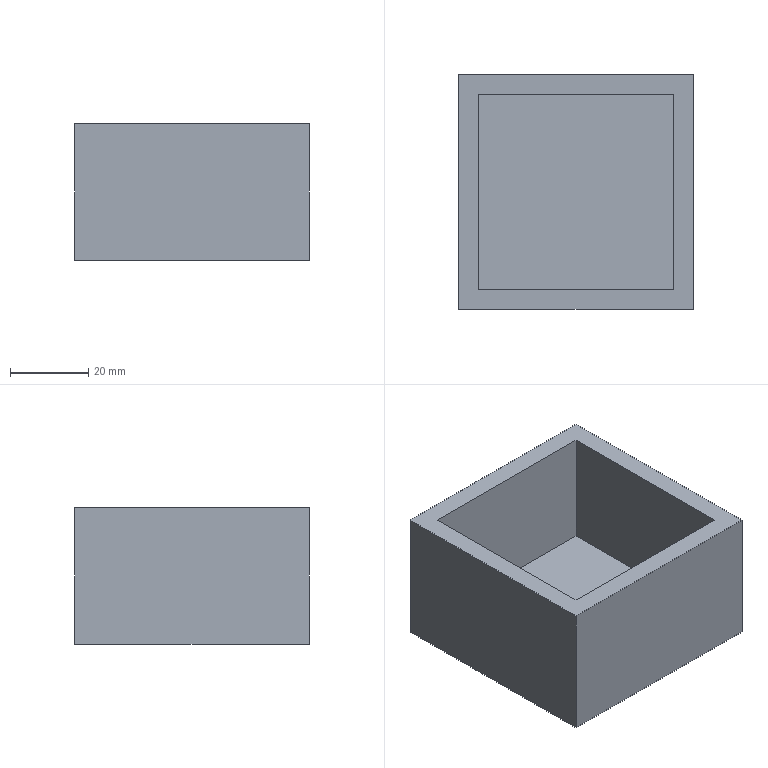Part | SolidWorks | features Extrusion 1, Shell 1 | 1 solid | 11 faces | box 60 x 60 x 35 mm | volume 51000 mm3 | plane 11
STEP:
#1=CARTESIAN_POINT('',(-58.,-30.,0.));
#2=VERTEX_POINT('',#1);
#3=CARTESIAN_POINT('',(-58.,30.,0.));
#4=VERTEX_POINT('',#3);
#5=CARTESIAN_POINT('',(-58.,30.,0.));
#6=DIRECTION('',(0.,1.,0.));
#7=VECTOR('',#6,1000.);
#8=LINE('',#5,#7);
#9=EDGE_CURVE('',#2,#4,#8,.T.);
#10=ORIENTED_EDGE('',*,*,#9,.T.);
#11=CARTESIAN_POINT('',(-58.,30.,35.));
#12=VERTEX_POINT('',#11);
#13=CARTESIAN_POINT('',(-58.,30.,35.));
#14=DIRECTION('',(0.,0.,-1.));
#15=VECTOR('',#14,1000.);
#16=LINE('',#13,#15);
#17=EDGE_CURVE('',#12,#4,#16,.T.);
#18=ORIENTED_EDGE('',*,*,#17,.F.);
#19=CARTESIAN_POINT('',(-58.,-30.,35.));
#20=VERTEX_POINT('',#19);
#21=CARTESIAN_POINT('',(-58.,30.,35.));
#22=DIRECTION('',(0.,1.,0.));
#23=VECTOR('',#22,1000.);
#24=LINE('',#21,#23);
#25=EDGE_CURVE('',#20,#12,#24,.T.);
#26=ORIENTED_EDGE('',*,*,#25,.F.);
#27=CARTESIAN_POINT('',(-58.,-30.,35.));
#28=DIRECTION('',(0.,0.,-1.));
#29=VECTOR('',#28,1000.);
#30=LINE('',#27,#29);
#31=EDGE_CURVE('',#20,#2,#30,.T.);
#32=ORIENTED_EDGE('',*,*,#31,.T.);
#33=EDGE_LOOP('',(#10,#18,#26,#32));
#34=FACE_OUTER_BOUND('',#33,.T.);
#35=CARTESIAN_POINT('',(-58.,30.,35.));
#36=DIRECTION('',(-1.,0.,0.));
#37=DIRECTION('',(0.,-1.,0.));
#38=AXIS2_PLACEMENT_3D('',#35,#36,#37);
#39=PLANE('',#38);
#40=ADVANCED_FACE('',(#34),#39,.F.);
#41=CARTESIAN_POINT('',(-118.,30.,0.));
#42=VERTEX_POINT('',#41);
#43=CARTESIAN_POINT('',(-118.,30.,0.));
#44=DIRECTION('',(-1.,0.,0.));
#45=VECTOR('',#44,1000.);
#46=LINE('',#43,#45);
#47=EDGE_CURVE('',#4,#42,#46,.T.);
#48=ORIENTED_EDGE('',*,*,#47,.T.);
#49=CARTESIAN_POINT('',(-118.,30.,35.));
#50=VERTEX_POINT('',#49);
#51=CARTESIAN_POINT('',(-118.,30.,35.));
#52=DIRECTION('',(0.,0.,-1.));
#53=VECTOR('',#52,1000.);
#54=LINE('',#51,#53);
#55=EDGE_CURVE('',#50,#42,#54,.T.);
#56=ORIENTED_EDGE('',*,*,#55,.F.);
#57=CARTESIAN_POINT('',(-118.,30.,35.));
#58=DIRECTION('',(-1.,0.,0.));
#59=VECTOR('',#58,1000.);
#60=LINE('',#57,#59);
#61=EDGE_CURVE('',#12,#50,#60,.T.);
#62=ORIENTED_EDGE('',*,*,#61,.F.);
#63=ORIENTED_EDGE('',*,*,#17,.T.);
#64=EDGE_LOOP('',(#48,#56,#62,#63));
#65=FACE_OUTER_BOUND('',#64,.T.);
#66=CARTESIAN_POINT('',(-118.,30.,35.));
#67=DIRECTION('',(0.,-1.,0.));
#68=DIRECTION('',(0.,0.,-1.));
#69=AXIS2_PLACEMENT_3D('',#66,#67,#68);
#70=PLANE('',#69);
#71=ADVANCED_FACE('',(#65),#70,.F.);
#72=CARTESIAN_POINT('',(-118.,-30.,0.));
#73=VERTEX_POINT('',#72);
#74=CARTESIAN_POINT('',(-118.,30.,0.));
#75=DIRECTION('',(0.,-1.,0.));
#76=VECTOR('',#75,1000.);
#77=LINE('',#74,#76);
#78=EDGE_CURVE('',#42,#73,#77,.T.);
#79=ORIENTED_EDGE('',*,*,#78,.T.);
#80=CARTESIAN_POINT('',(-118.,-30.,35.));
#81=VERTEX_POINT('',#80);
#82=CARTESIAN_POINT('',(-118.,-30.,35.));
#83=DIRECTION('',(0.,0.,-1.));
#84=VECTOR('',#83,1000.);
#85=LINE('',#82,#84);
#86=EDGE_CURVE('',#81,#73,#85,.T.);
#87=ORIENTED_EDGE('',*,*,#86,.F.);
#88=CARTESIAN_POINT('',(-118.,30.,35.));
#89=DIRECTION('',(0.,-1.,0.));
#90=VECTOR('',#89,1000.);
#91=LINE('',#88,#90);
#92=EDGE_CURVE('',#50,#81,#91,.T.);
#93=ORIENTED_EDGE('',*,*,#92,.F.);
#94=ORIENTED_EDGE('',*,*,#55,.T.);
#95=EDGE_LOOP('',(#79,#87,#93,#94));
#96=FACE_OUTER_BOUND('',#95,.T.);
#97=CARTESIAN_POINT('',(-118.,30.,35.));
#98=DIRECTION('',(1.,0.,0.));
#99=DIRECTION('',(0.,1.,0.));
#100=AXIS2_PLACEMENT_3D('',#97,#98,#99);
#101=PLANE('',#100);
#102=ADVANCED_FACE('',(#96),#101,.F.);
#103=CARTESIAN_POINT('',(-118.,-30.,0.));
#104=DIRECTION('',(1.,0.,0.));
#105=VECTOR('',#104,1000.);
#106=LINE('',#103,#105);
#107=EDGE_CURVE('',#73,#2,#106,.T.);
#108=ORIENTED_EDGE('',*,*,#107,.T.);
#109=ORIENTED_EDGE('',*,*,#31,.F.);
#110=CARTESIAN_POINT('',(-118.,-30.,35.));
#111=DIRECTION('',(1.,0.,0.));
#112=VECTOR('',#111,1000.);
#113=LINE('',#110,#112);
#114=EDGE_CURVE('',#81,#20,#113,.T.);
#115=ORIENTED_EDGE('',*,*,#114,.F.);
#116=ORIENTED_EDGE('',*,*,#86,.T.);
#117=EDGE_LOOP('',(#108,#109,#115,#116));
#118=FACE_OUTER_BOUND('',#117,.T.);
#119=CARTESIAN_POINT('',(-118.,-30.,35.));
#120=DIRECTION('',(0.,1.,0.));
#121=DIRECTION('',(0.,0.,1.));
#122=AXIS2_PLACEMENT_3D('',#119,#120,#121);
#123=PLANE('',#122);
#124=ADVANCED_FACE('',(#118),#123,.F.);
#125=CARTESIAN_POINT('',(-63.,-25.,35.));
#126=VERTEX_POINT('',#125);
#127=CARTESIAN_POINT('',(-63.,25.,35.));
#128=VERTEX_POINT('',#127);
#129=CARTESIAN_POINT('',(-63.,30.,35.));
#130=DIRECTION('',(0.,1.,0.));
#131=VECTOR('',#130,1000.);
#132=LINE('',#129,#131);
#133=EDGE_CURVE('',#126,#128,#132,.T.);
#134=ORIENTED_EDGE('',*,*,#133,.F.);
#135=CARTESIAN_POINT('',(-113.,-25.,35.));
#136=VERTEX_POINT('',#135);
#137=CARTESIAN_POINT('',(-118.,-25.,35.));
#138=DIRECTION('',(1.,0.,0.));
#139=VECTOR('',#138,1000.);
#140=LINE('',#137,#139);
#141=EDGE_CURVE('',#136,#126,#140,.T.);
#142=ORIENTED_EDGE('',*,*,#141,.F.);
#143=CARTESIAN_POINT('',(-113.,25.,35.));
#144=VERTEX_POINT('',#143);
#145=CARTESIAN_POINT('',(-113.,30.,35.));
#146=DIRECTION('',(0.,-1.,0.));
#147=VECTOR('',#146,1000.);
#148=LINE('',#145,#147);
#149=EDGE_CURVE('',#144,#136,#148,.T.);
#150=ORIENTED_EDGE('',*,*,#149,.F.);
#151=CARTESIAN_POINT('',(-118.,25.,35.));
#152=DIRECTION('',(-1.,0.,0.));
#153=VECTOR('',#152,1000.);
#154=LINE('',#151,#153);
#155=EDGE_CURVE('',#128,#144,#154,.T.);
#156=ORIENTED_EDGE('',*,*,#155,.F.);
#157=EDGE_LOOP('',(#134,#142,#150,#156));
#158=FACE_BOUND('',#157,.T.);
#159=ORIENTED_EDGE('',*,*,#25,.T.);
#160=ORIENTED_EDGE('',*,*,#61,.T.);
#161=ORIENTED_EDGE('',*,*,#92,.T.);
#162=ORIENTED_EDGE('',*,*,#114,.T.);
#163=EDGE_LOOP('',(#159,#160,#161,#162));
#164=FACE_OUTER_BOUND('',#163,.T.);
#165=CARTESIAN_POINT('',(0.,0.,35.));
#166=DIRECTION('',(0.,0.,1.));
#167=DIRECTION('',(1.,0.,0.));
#168=AXIS2_PLACEMENT_3D('',#165,#166,#167);
#169=PLANE('',#168);
#170=ADVANCED_FACE('',(#158,#164),#169,.T.);
#171=ORIENTED_EDGE('',*,*,#9,.F.);
#172=ORIENTED_EDGE('',*,*,#107,.F.);
#173=ORIENTED_EDGE('',*,*,#78,.F.);
#174=ORIENTED_EDGE('',*,*,#47,.F.);
#175=EDGE_LOOP('',(#171,#172,#173,#174));
#176=FACE_OUTER_BOUND('',#175,.T.);
#177=CARTESIAN_POINT('',(0.,0.,0.));
#178=DIRECTION('',(0.,0.,1.));
#179=DIRECTION('',(1.,0.,0.));
#180=AXIS2_PLACEMENT_3D('',#177,#178,#179);
#181=PLANE('',#180);
#182=ADVANCED_FACE('',(#176),#181,.F.);
#183=CARTESIAN_POINT('',(-63.,-25.,5.));
#184=VERTEX_POINT('',#183);
#185=CARTESIAN_POINT('',(-63.,25.,5.));
#186=VERTEX_POINT('',#185);
#187=CARTESIAN_POINT('',(-63.,30.,5.));
#188=DIRECTION('',(0.,1.,0.));
#189=VECTOR('',#188,1000.);
#190=LINE('',#187,#189);
#191=EDGE_CURVE('',#184,#186,#190,.T.);
#192=ORIENTED_EDGE('',*,*,#191,.F.);
#193=CARTESIAN_POINT('',(-63.,-25.,35.));
#194=DIRECTION('',(0.,0.,-1.));
#195=VECTOR('',#194,1000.);
#196=LINE('',#193,#195);
#197=EDGE_CURVE('',#126,#184,#196,.T.);
#198=ORIENTED_EDGE('',*,*,#197,.F.);
#199=ORIENTED_EDGE('',*,*,#133,.T.);
#200=CARTESIAN_POINT('',(-63.,25.,35.));
#201=DIRECTION('',(0.,0.,-1.));
#202=VECTOR('',#201,1000.);
#203=LINE('',#200,#202);
#204=EDGE_CURVE('',#128,#186,#203,.T.);
#205=ORIENTED_EDGE('',*,*,#204,.T.);
#206=EDGE_LOOP('',(#192,#198,#199,#205));
#207=FACE_OUTER_BOUND('',#206,.T.);
#208=CARTESIAN_POINT('',(-63.,30.,35.));
#209=DIRECTION('',(-1.,0.,0.));
#210=DIRECTION('',(0.,-1.,0.));
#211=AXIS2_PLACEMENT_3D('',#208,#209,#210);
#212=PLANE('',#211);
#213=ADVANCED_FACE('',(#207),#212,.T.);
#214=CARTESIAN_POINT('',(-113.,25.,5.));
#215=VERTEX_POINT('',#214);
#216=CARTESIAN_POINT('',(-118.,25.,5.));
#217=DIRECTION('',(-1.,0.,0.));
#218=VECTOR('',#217,1000.);
#219=LINE('',#216,#218);
#220=EDGE_CURVE('',#186,#215,#219,.T.);
#221=ORIENTED_EDGE('',*,*,#220,.F.);
#222=ORIENTED_EDGE('',*,*,#204,.F.);
#223=ORIENTED_EDGE('',*,*,#155,.T.);
#224=CARTESIAN_POINT('',(-113.,25.,35.));
#225=DIRECTION('',(0.,0.,-1.));
#226=VECTOR('',#225,1000.);
#227=LINE('',#224,#226);
#228=EDGE_CURVE('',#144,#215,#227,.T.);
#229=ORIENTED_EDGE('',*,*,#228,.T.);
#230=EDGE_LOOP('',(#221,#222,#223,#229));
#231=FACE_OUTER_BOUND('',#230,.T.);
#232=CARTESIAN_POINT('',(-118.,25.,35.));
#233=DIRECTION('',(0.,-1.,0.));
#234=DIRECTION('',(0.,0.,-1.));
#235=AXIS2_PLACEMENT_3D('',#232,#233,#234);
#236=PLANE('',#235);
#237=ADVANCED_FACE('',(#231),#236,.T.);
#238=CARTESIAN_POINT('',(-113.,-25.,5.));
#239=VERTEX_POINT('',#238);
#240=CARTESIAN_POINT('',(-113.,30.,5.));
#241=DIRECTION('',(0.,-1.,0.));
#242=VECTOR('',#241,1000.);
#243=LINE('',#240,#242);
#244=EDGE_CURVE('',#215,#239,#243,.T.);
#245=ORIENTED_EDGE('',*,*,#244,.F.);
#246=ORIENTED_EDGE('',*,*,#228,.F.);
#247=ORIENTED_EDGE('',*,*,#149,.T.);
#248=CARTESIAN_POINT('',(-113.,-25.,35.));
#249=DIRECTION('',(0.,0.,-1.));
#250=VECTOR('',#249,1000.);
#251=LINE('',#248,#250);
#252=EDGE_CURVE('',#136,#239,#251,.T.);
#253=ORIENTED_EDGE('',*,*,#252,.T.);
#254=EDGE_LOOP('',(#245,#246,#247,#253));
#255=FACE_OUTER_BOUND('',#254,.T.);
#256=CARTESIAN_POINT('',(-113.,30.,35.));
#257=DIRECTION('',(1.,0.,0.));
#258=DIRECTION('',(0.,1.,0.));
#259=AXIS2_PLACEMENT_3D('',#256,#257,#258);
#260=PLANE('',#259);
#261=ADVANCED_FACE('',(#255),#260,.T.);
#262=CARTESIAN_POINT('',(-118.,-25.,5.));
#263=DIRECTION('',(1.,0.,0.));
#264=VECTOR('',#263,1000.);
#265=LINE('',#262,#264);
#266=EDGE_CURVE('',#239,#184,#265,.T.);
#267=ORIENTED_EDGE('',*,*,#266,.F.);
#268=ORIENTED_EDGE('',*,*,#252,.F.);
#269=ORIENTED_EDGE('',*,*,#141,.T.);
#270=ORIENTED_EDGE('',*,*,#197,.T.);
#271=EDGE_LOOP('',(#267,#268,#269,#270));
#272=FACE_OUTER_BOUND('',#271,.T.);
#273=CARTESIAN_POINT('',(-118.,-25.,35.));
#274=DIRECTION('',(0.,1.,0.));
#275=DIRECTION('',(0.,0.,1.));
#276=AXIS2_PLACEMENT_3D('',#273,#274,#275);
#277=PLANE('',#276);
#278=ADVANCED_FACE('',(#272),#277,.T.);
#279=ORIENTED_EDGE('',*,*,#191,.T.);
#280=ORIENTED_EDGE('',*,*,#220,.T.);
#281=ORIENTED_EDGE('',*,*,#244,.T.);
#282=ORIENTED_EDGE('',*,*,#266,.T.);
#283=EDGE_LOOP('',(#279,#280,#281,#282));
#284=FACE_OUTER_BOUND('',#283,.T.);
#285=CARTESIAN_POINT('',(0.,0.,5.));
#286=DIRECTION('',(0.,0.,1.));
#287=DIRECTION('',(1.,0.,0.));
#288=AXIS2_PLACEMENT_3D('',#285,#286,#287);
#289=PLANE('',#288);
#290=ADVANCED_FACE('',(#284),#289,.T.);
#291=CLOSED_SHELL('',(#40,#71,#102,#124,#170,#182,#213,#237,#261,#278,#290));
#292=MANIFOLD_SOLID_BREP('',#291);
#293=CARTESIAN_POINT('',(0.,0.,0.));
#294=DIRECTION('',(0.,0.,1.));
#295=DIRECTION('',(1.,0.,0.));
#296=AXIS2_PLACEMENT_3D('',#293,#294,#295);
#297=(LENGTH_UNIT()NAMED_UNIT(*)SI_UNIT(.MILLI.,.METRE.));
#298=UNCERTAINTY_MEASURE_WITH_UNIT(LENGTH_MEASURE(0.00001),#297,'','');
#299=(NAMED_UNIT(*)PLANE_ANGLE_UNIT()SI_UNIT($,.RADIAN.));
#300=(NAMED_UNIT(*)SI_UNIT($,.STERADIAN.)SOLID_ANGLE_UNIT());
#301=(GEOMETRIC_REPRESENTATION_CONTEXT(3)GLOBAL_UNCERTAINTY_ASSIGNED_CONTEXT((#298))GLOBAL_UNIT_ASSIGNED_CONTEXT((#297,#299,#300))REPRESENTATION_CONTEXT('',''));
#302=ADVANCED_BREP_SHAPE_REPRESENTATION('',(#292,#296),#301);